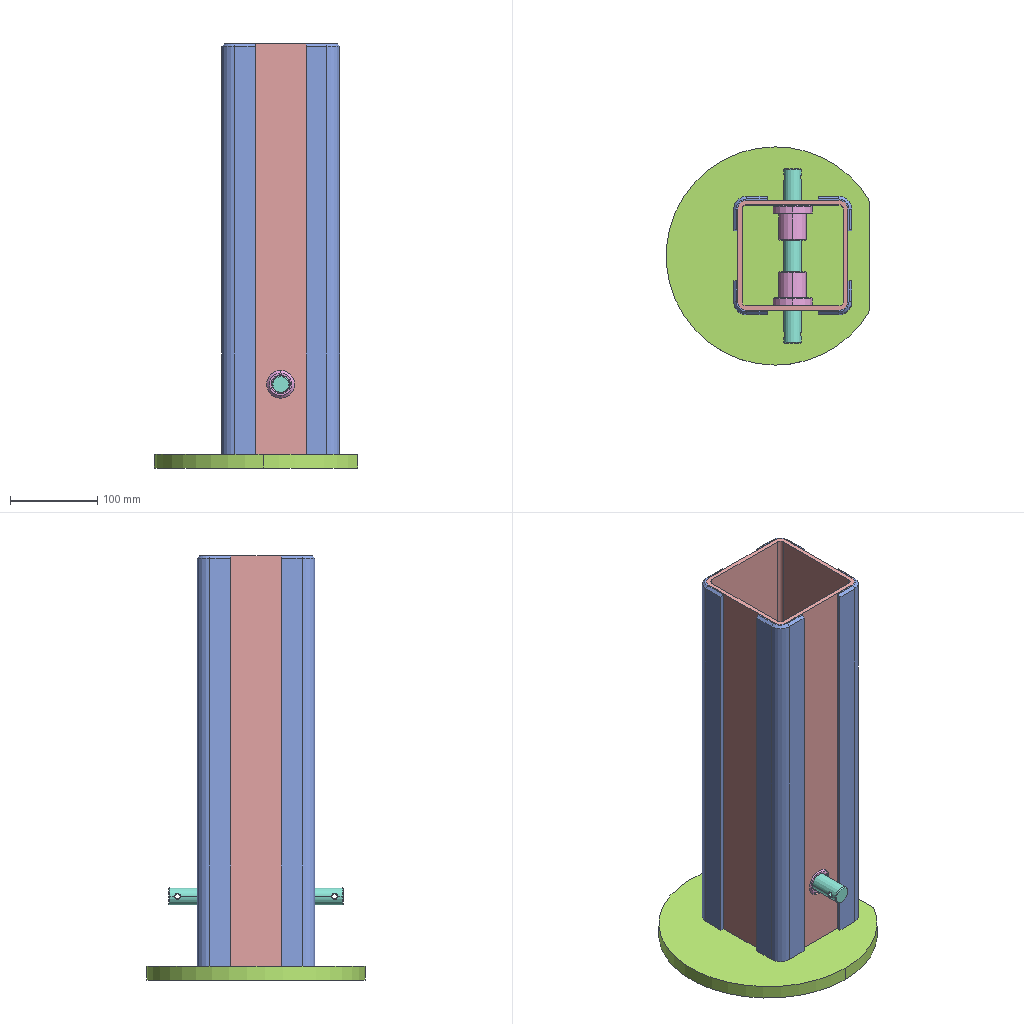Assembly | SolidWorks | 5 different items | 9 placed | box 233 x 250 x 486 mm
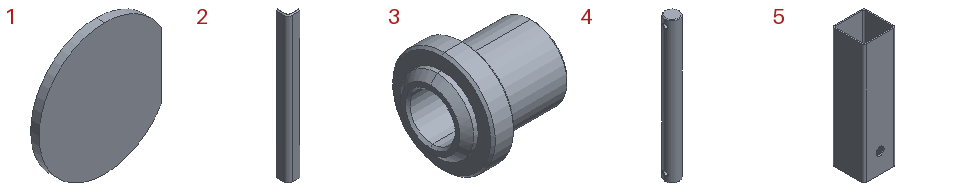Parts list (item | quantity | size | volume | features):
1 | x1 | 233 x 16 x 250 mm | 762244 mm3 | features FlatPattern 1, SMBaseFlange 1, SheetMetal 1
2 | x4 | 38.5 x 38.5 x 470 mm | 141906 mm3 | features Chamfer 1, FlatPattern 1, SMBaseFlange 1, SheetMetal 1
3 | x2 | 45 x 45 x 45 mm | 29238 mm3 | features Chamfer 2, Revolution 1
4 | x1 | 20 x 20 x 200 mm | 61631 mm3 | features Chamfer 2, Extrusion 1, ICE 1
5 | x1 | 126 x 126 x 470 mm | 1099099 mm3 | features Attribute 1, Extrusion 1, ICE 1
Mates (type | each side: item.copy, entity, surface, feature):
Coincident | 5.1 face plane Boss-Extrude1 | 2.1 face plane Base-Flange1 | 3 times
Coincident | 5.1 face plane Boss-Extrude1 | 2.2 face plane Base-Flange1 | 3 times
Coincident | 5.1 face plane Boss-Extrude1 | 2.3 face plane Base-Flange1 | 3 times
Coincident | 5.1 face plane Boss-Extrude1 | 2.4 face plane Base-Flange1 | 3 times
Coincident | 5.1 face plane Boss-Extrude1 | 1.1 face plane Base-Flange1
Coincident | 5.1 plane | 1.1 plane
DistanceDim | 5.1 plane | 1.1 plane
Concentric | 5.1 face cylinder Cut-Extrude1 | 3.1 face cylinder Revolve1
Coincident | 5.1 face plane Boss-Extrude1 | 3.1 face plane Revolve1
Concentric | 5.1 face cylinder Cut-Extrude1 | 3.2 face cylinder Revolve1
Coincident | 5.1 face plane Boss-Extrude1 | 3.2 face plane Revolve1
Concentric | 3.1 face cylinder Revolve1 | 4.1 face cylinder Boss-Extrude1
DistanceDim | 5.1 face plane Boss-Extrude1 | 4.1 face plane Boss-Extrude1
Parallel | 4.1 plane | assembly plane | 3 times